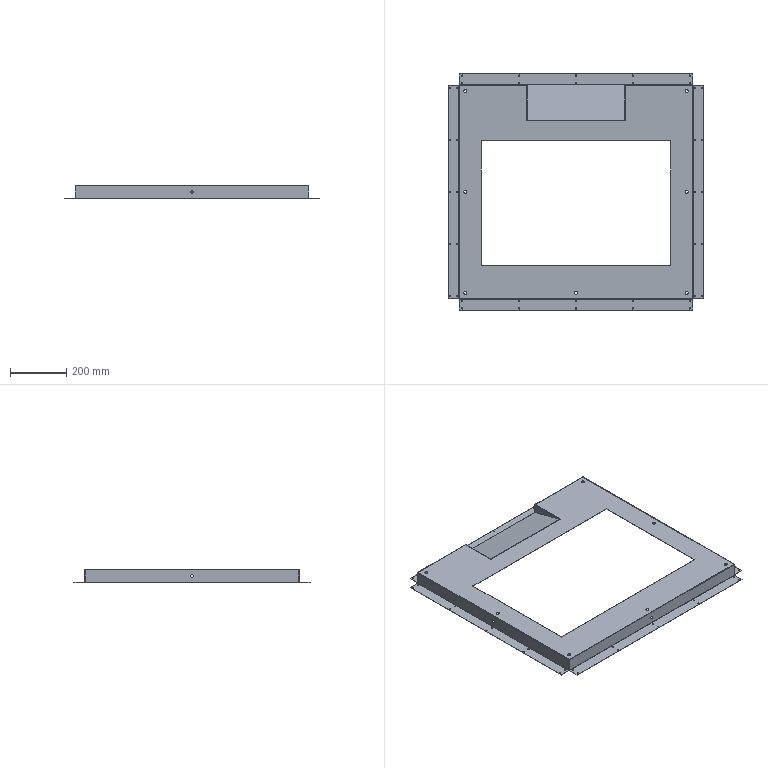Part | 2 solids | 204 faces | box 913 x 843 x 48 mm | volume 603104 mm3 | cylinder 122 | plane 70 | spline 12 | commonest cylinder face diameters 4.2 x80 11 x14 0.4 x11 2.4 x11 10 x6